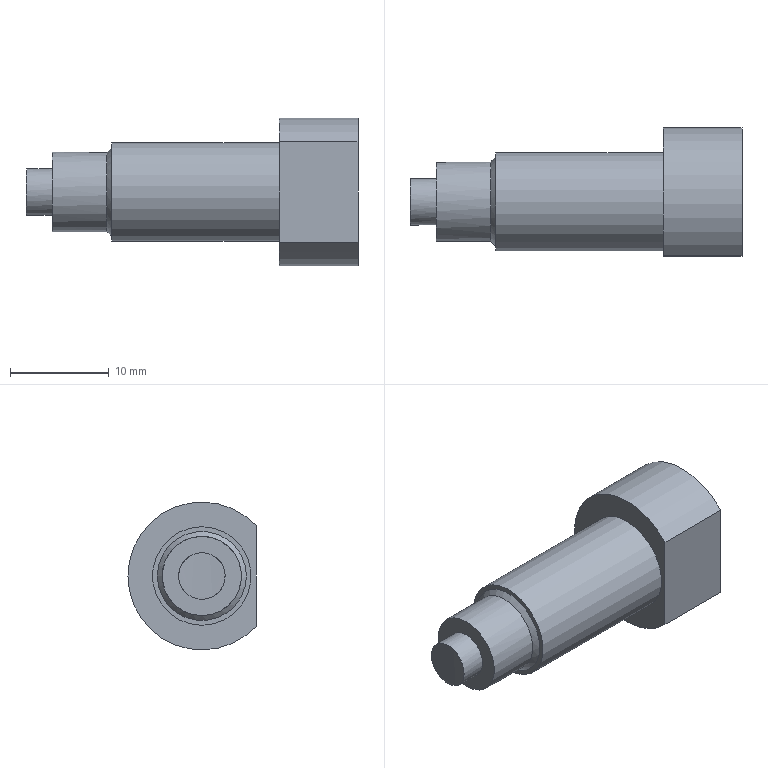Part | NX | features solid 2 | 1 solid | 11 faces | box 33.693 x 13 x 15 mm | volume 2992 mm3 | plane 5 | cylinder 4 | cone 2 | commonest cylinder face diameters 4.723 x1 8.04 x1 10 x1 15 x1
STEP:
#1=CARTESIAN_POINT('',(72.275,-5.5,-7.783));
#2=VERTEX_POINT('',#1);
#3=CARTESIAN_POINT('',(72.275,-5.5,-17.981));
#4=VERTEX_POINT('',#3);
#5=CARTESIAN_POINT('',(72.275,0.,-12.882));
#6=DIRECTION('',(1.,0.,0.));
#7=DIRECTION('',(0.,0.,-1.));
#8=AXIS2_PLACEMENT_3D('',#5,#6,#7);
#9=CIRCLE('',#8,7.5);
#10=EDGE_CURVE('',#2,#4,#9,.F.);
#11=ORIENTED_EDGE('',*,*,#10,.F.);
#12=CARTESIAN_POINT('',(80.275,-5.5,-7.783));
#13=VERTEX_POINT('',#12);
#14=CARTESIAN_POINT('',(80.275,-5.5,-7.783));
#15=DIRECTION('',(-1.,0.,0.));
#16=VECTOR('',#15,1000.);
#17=LINE('',#14,#16);
#18=EDGE_CURVE('',#2,#13,#17,.F.);
#19=ORIENTED_EDGE('',*,*,#18,.T.);
#20=CARTESIAN_POINT('',(80.275,-5.5,-17.981));
#21=VERTEX_POINT('',#20);
#22=CARTESIAN_POINT('',(80.275,0.,-12.882));
#23=DIRECTION('',(1.,0.,0.));
#24=DIRECTION('',(0.,0.,-1.));
#25=AXIS2_PLACEMENT_3D('',#22,#23,#24);
#26=CIRCLE('',#25,7.5);
#27=EDGE_CURVE('',#13,#21,#26,.F.);
#28=ORIENTED_EDGE('',*,*,#27,.T.);
#29=CARTESIAN_POINT('',(80.275,-5.5,-17.981));
#30=DIRECTION('',(-1.,0.,0.));
#31=VECTOR('',#30,1000.);
#32=LINE('',#29,#31);
#33=EDGE_CURVE('',#21,#4,#32,.T.);
#34=ORIENTED_EDGE('',*,*,#33,.T.);
#35=EDGE_LOOP('',(#11,#19,#28,#34));
#36=FACE_BOUND('',#35,.T.);
#37=CARTESIAN_POINT('',(80.275,0.,-12.882));
#38=DIRECTION('',(-1.,0.,0.));
#39=DIRECTION('',(0.,0.,1.));
#40=AXIS2_PLACEMENT_3D('',#37,#38,#39);
#41=CYLINDRICAL_SURFACE('',#40,7.5);
#42=ADVANCED_FACE('',(#36),#41,.T.);
#43=ORIENTED_EDGE('',*,*,#27,.F.);
#44=CARTESIAN_POINT('',(80.275,-5.5,-12.882));
#45=DIRECTION('',(0.,0.,-1.));
#46=VECTOR('',#45,1000.);
#47=LINE('',#44,#46);
#48=EDGE_CURVE('',#13,#21,#47,.T.);
#49=ORIENTED_EDGE('',*,*,#48,.T.);
#50=EDGE_LOOP('',(#43,#49));
#51=FACE_BOUND('',#50,.T.);
#52=CARTESIAN_POINT('',(80.275,0.,-24.942));
#53=DIRECTION('',(1.,0.,0.));
#54=DIRECTION('',(0.,0.,-1.));
#55=AXIS2_PLACEMENT_3D('',#52,#53,#54);
#56=PLANE('',#55);
#57=ADVANCED_FACE('',(#51),#56,.T.);
#58=CARTESIAN_POINT('',(72.275,0.,-17.882));
#59=VERTEX_POINT('',#58);
#60=CARTESIAN_POINT('',(72.275,0.,-12.882));
#61=DIRECTION('',(1.,0.,0.));
#62=DIRECTION('',(0.,0.,-1.));
#63=AXIS2_PLACEMENT_3D('',#60,#61,#62);
#64=CIRCLE('',#63,5.);
#65=EDGE_CURVE('',#59,#59,#64,.T.);
#66=ORIENTED_EDGE('',*,*,#65,.F.);
#67=EDGE_LOOP('',(#66));
#68=FACE_BOUND('',#67,.T.);
#69=CARTESIAN_POINT('',(55.275,0.,-17.882));
#70=VERTEX_POINT('',#69);
#71=CARTESIAN_POINT('',(55.275,0.,-12.882));
#72=DIRECTION('',(1.,0.,0.));
#73=DIRECTION('',(0.,0.,-1.));
#74=AXIS2_PLACEMENT_3D('',#71,#72,#73);
#75=CIRCLE('',#74,5.);
#76=EDGE_CURVE('',#70,#70,#75,.F.);
#77=ORIENTED_EDGE('',*,*,#76,.F.);
#78=EDGE_LOOP('',(#77));
#79=FACE_BOUND('',#78,.T.);
#80=CARTESIAN_POINT('',(-39.725,0.,-12.882));
#81=DIRECTION('',(1.,0.,0.));
#82=DIRECTION('',(0.,0.,-1.));
#83=AXIS2_PLACEMENT_3D('',#80,#81,#82);
#84=CYLINDRICAL_SURFACE('',#83,5.);
#85=ADVANCED_FACE('',(#68,#79),#84,.T.);
#86=CARTESIAN_POINT('',(49.245,0.,-10.521));
#87=VERTEX_POINT('',#86);
#88=CARTESIAN_POINT('',(49.245,0.,-12.882));
#89=DIRECTION('',(1.,0.,0.));
#90=DIRECTION('',(0.,0.,1.));
#91=AXIS2_PLACEMENT_3D('',#88,#89,#90);
#92=CIRCLE('',#91,2.362);
#93=EDGE_CURVE('',#87,#87,#92,.T.);
#94=ORIENTED_EDGE('',*,*,#93,.T.);
#95=EDGE_LOOP('',(#94));
#96=FACE_BOUND('',#95,.T.);
#97=CARTESIAN_POINT('',(49.245,0.,-16.902));
#98=VERTEX_POINT('',#97);
#99=CARTESIAN_POINT('',(49.245,0.,-12.882));
#100=DIRECTION('',(1.,0.,0.));
#101=DIRECTION('',(0.,0.,-1.));
#102=AXIS2_PLACEMENT_3D('',#99,#100,#101);
#103=CIRCLE('',#102,4.02);
#104=EDGE_CURVE('',#98,#98,#103,.F.);
#105=ORIENTED_EDGE('',*,*,#104,.T.);
#106=EDGE_LOOP('',(#105));
#107=FACE_BOUND('',#106,.T.);
#108=CARTESIAN_POINT('',(49.245,0.,-24.942));
#109=DIRECTION('',(1.,0.,0.));
#110=DIRECTION('',(0.,0.,-1.));
#111=AXIS2_PLACEMENT_3D('',#108,#109,#110);
#112=PLANE('',#111);
#113=ADVANCED_FACE('',(#96,#107),#112,.F.);
#114=CARTESIAN_POINT('',(54.773,4.02,-12.882));
#115=VERTEX_POINT('',#114);
#116=CARTESIAN_POINT('',(54.773,0.,-12.882));
#117=DIRECTION('',(1.,0.,0.));
#118=DIRECTION('',(0.,1.,0.));
#119=AXIS2_PLACEMENT_3D('',#116,#117,#118);
#120=CIRCLE('',#119,4.02);
#121=EDGE_CURVE('',#115,#115,#120,.T.);
#122=ORIENTED_EDGE('',*,*,#121,.F.);
#123=EDGE_LOOP('',(#122));
#124=FACE_BOUND('',#123,.T.);
#125=ORIENTED_EDGE('',*,*,#104,.F.);
#126=EDGE_LOOP('',(#125));
#127=FACE_BOUND('',#126,.T.);
#128=CARTESIAN_POINT('',(55.275,0.,-12.882));
#129=DIRECTION('',(1.,0.,0.));
#130=DIRECTION('',(0.,0.,-1.));
#131=AXIS2_PLACEMENT_3D('',#128,#129,#130);
#132=CYLINDRICAL_SURFACE('',#131,4.02);
#133=ADVANCED_FACE('',(#124,#127),#132,.T.);
#134=ORIENTED_EDGE('',*,*,#121,.T.);
#135=EDGE_LOOP('',(#134));
#136=FACE_BOUND('',#135,.T.);
#137=CARTESIAN_POINT('',(55.275,4.522,-12.882));
#138=VERTEX_POINT('',#137);
#139=CARTESIAN_POINT('',(55.275,0.,-12.882));
#140=DIRECTION('',(1.,0.,0.));
#141=DIRECTION('',(0.,1.,0.));
#142=AXIS2_PLACEMENT_3D('',#139,#140,#141);
#143=CIRCLE('',#142,4.522);
#144=EDGE_CURVE('',#138,#138,#143,.T.);
#145=ORIENTED_EDGE('',*,*,#144,.F.);
#146=EDGE_LOOP('',(#145));
#147=FACE_BOUND('',#146,.T.);
#148=CARTESIAN_POINT('',(55.024,0.,-12.882));
#149=DIRECTION('',(1.,0.,0.));
#150=DIRECTION('',(0.,0.,1.));
#151=AXIS2_PLACEMENT_3D('',#148,#149,#150);
#152=CONICAL_SURFACE('',#151,4.271,0.7854);
#153=ADVANCED_FACE('',(#136,#147),#152,.T.);
#154=ORIENTED_EDGE('',*,*,#76,.T.);
#155=EDGE_LOOP('',(#154));
#156=FACE_BOUND('',#155,.T.);
#157=ORIENTED_EDGE('',*,*,#144,.T.);
#158=EDGE_LOOP('',(#157));
#159=FACE_BOUND('',#158,.T.);
#160=CARTESIAN_POINT('',(55.275,0.,-24.942));
#161=DIRECTION('',(1.,0.,0.));
#162=DIRECTION('',(0.,0.,-1.));
#163=AXIS2_PLACEMENT_3D('',#160,#161,#162);
#164=PLANE('',#163);
#165=ADVANCED_FACE('',(#156,#159),#164,.F.);
#166=ORIENTED_EDGE('',*,*,#93,.F.);
#167=EDGE_LOOP('',(#166));
#168=FACE_BOUND('',#167,.T.);
#169=CARTESIAN_POINT('',(46.623,0.,-15.244));
#170=VERTEX_POINT('',#169);
#171=CARTESIAN_POINT('',(46.598,1.853,-14.732));
#172=CARTESIAN_POINT('',(46.636,-0.0004769,-15.5));
#173=CARTESIAN_POINT('',(46.598,-1.851,-14.732));
#174=CARTESIAN_POINT('',(46.569,-2.617,-12.884));
#175=CARTESIAN_POINT('',(46.63,-1.852,-11.032));
#176=CARTESIAN_POINT('',(46.681,-0.0003832,-10.265));
#177=CARTESIAN_POINT('',(46.63,1.848,-11.03));
#178=CARTESIAN_POINT('',(46.569,2.617,-12.879));
#179=CARTESIAN_POINT('',(46.598,1.853,-14.732));
#180=CARTESIAN_POINT('',(46.636,-0.0004769,-15.5));
#181=CARTESIAN_POINT('',(46.598,-1.851,-14.732));
#182=B_SPLINE_CURVE_WITH_KNOTS('',3,(#171,#172,#173,#174,#175,#176,#177,#178,#179,#180,#181),.UNSPECIFIED.,.T.,.F.,(1,1,1,1,1,1,1,1,1,1,1,1,1,1,1),(-0.005538,-0.003692,-0.001846,0.,0.001846,0.003692,0.005538,0.007384,0.00923,0.01108,0.01292,0.01477,0.01661,0.01846,0.02031),.UNSPECIFIED.);
#183=EDGE_CURVE('',#170,#170,#182,.T.);
#184=ORIENTED_EDGE('',*,*,#183,.F.);
#185=EDGE_LOOP('',(#184));
#186=FACE_BOUND('',#185,.T.);
#187=CARTESIAN_POINT('',(55.275,0.,-12.882));
#188=DIRECTION('',(1.,0.,0.));
#189=DIRECTION('',(0.,0.,-1.));
#190=AXIS2_PLACEMENT_3D('',#187,#188,#189);
#191=CYLINDRICAL_SURFACE('',#190,2.362);
#192=ADVANCED_FACE('',(#168,#186),#191,.T.);
#193=ORIENTED_EDGE('',*,*,#183,.T.);
#194=EDGE_LOOP('',(#193));
#195=FACE_BOUND('',#194,.T.);
#196=CARTESIAN_POINT('',(0.,0.,6.217));
#197=DIRECTION('',(0.,0.,1.));
#198=DIRECTION('',(0.,1.,0.));
#199=AXIS2_PLACEMENT_3D('',#196,#197,#198);
#200=CONICAL_SURFACE('',#199,46.81,0.008727);
#201=ADVANCED_FACE('',(#195),#200,.F.);
#202=CARTESIAN_POINT('',(72.275,-5.5,-12.882));
#203=DIRECTION('',(0.,0.,1.));
#204=VECTOR('',#203,1000.);
#205=LINE('',#202,#204);
#206=EDGE_CURVE('',#2,#4,#205,.F.);
#207=ORIENTED_EDGE('',*,*,#206,.F.);
#208=ORIENTED_EDGE('',*,*,#10,.T.);
#209=EDGE_LOOP('',(#207,#208));
#210=FACE_BOUND('',#209,.T.);
#211=ORIENTED_EDGE('',*,*,#65,.T.);
#212=EDGE_LOOP('',(#211));
#213=FACE_BOUND('',#212,.T.);
#214=CARTESIAN_POINT('',(72.275,0.,-12.882));
#215=DIRECTION('',(1.,0.,0.));
#216=DIRECTION('',(0.,0.,-1.));
#217=AXIS2_PLACEMENT_3D('',#214,#215,#216);
#218=PLANE('',#217);
#219=ADVANCED_FACE('',(#210,#213),#218,.F.);
#220=ORIENTED_EDGE('',*,*,#206,.T.);
#221=ORIENTED_EDGE('',*,*,#33,.F.);
#222=ORIENTED_EDGE('',*,*,#48,.F.);
#223=ORIENTED_EDGE('',*,*,#18,.F.);
#224=EDGE_LOOP('',(#220,#221,#222,#223));
#225=FACE_BOUND('',#224,.T.);
#226=CARTESIAN_POINT('',(76.275,-5.5,-12.882));
#227=DIRECTION('',(0.,-1.,0.));
#228=DIRECTION('',(1.,0.,0.));
#229=AXIS2_PLACEMENT_3D('',#226,#227,#228);
#230=PLANE('',#229);
#231=ADVANCED_FACE('',(#225),#230,.T.);
#232=CLOSED_SHELL('',(#42,#57,#85,#113,#133,#153,#165,#192,#201,#219,#231));
#233=MANIFOLD_SOLID_BREP('',#232);
#234=(LENGTH_UNIT()NAMED_UNIT(*)SI_UNIT(.MILLI.,.METRE.));
#235=UNCERTAINTY_MEASURE_WITH_UNIT(LENGTH_MEASURE(0.0508),#234,'','');
#236=(NAMED_UNIT(*)PLANE_ANGLE_UNIT()SI_UNIT($,.RADIAN.));
#237=(NAMED_UNIT(*)SI_UNIT($,.STERADIAN.)SOLID_ANGLE_UNIT());
#238=(GEOMETRIC_REPRESENTATION_CONTEXT(3)GLOBAL_UNCERTAINTY_ASSIGNED_CONTEXT((#235))GLOBAL_UNIT_ASSIGNED_CONTEXT((#234,#236,#237))REPRESENTATION_CONTEXT('',''));
#239=ADVANCED_BREP_SHAPE_REPRESENTATION('',(#233),#238);